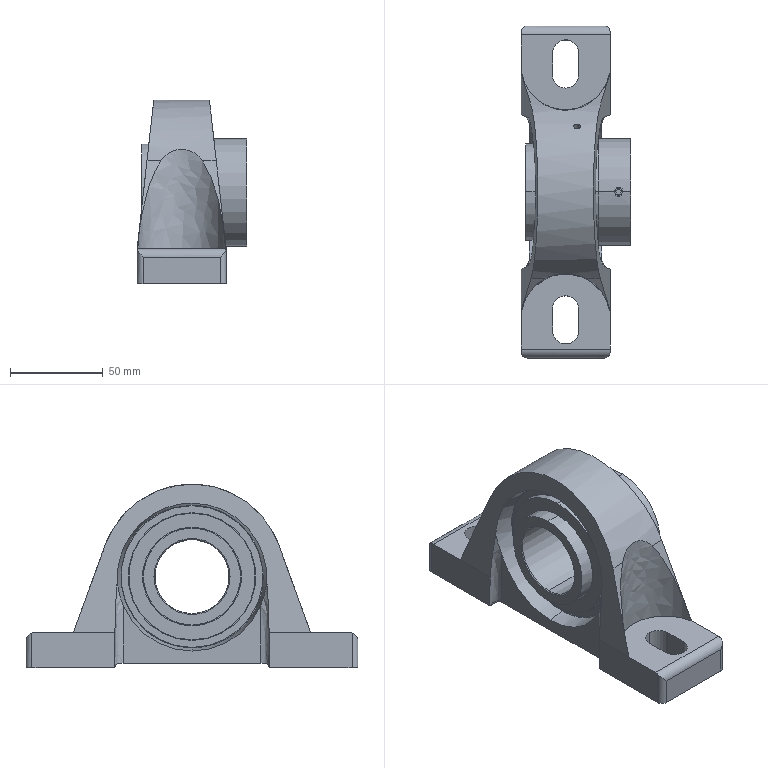Part | SolidWorks | 14 solids | 196 faces | box 59.2 x 179 x 99 mm | volume 299518 mm3 | spline 104 | plane 63 | cylinder 29 | commonest cylinder face diameters 6.4 x4 52.3 x4 66.3 x4 68.3 x4 70.89 x4 5 x2